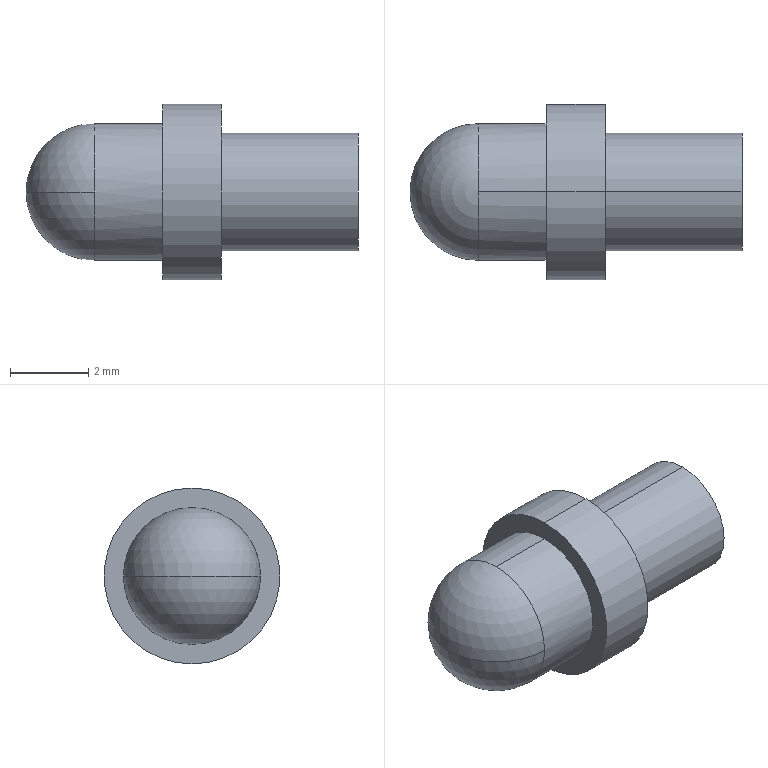Part | STEP file | RSR-PB107_grease_nipple_joint(2)^SRS15MUU-220LM-G10_Buffer motion shaft | 1 solid | 11 faces | box 8.5 x 4.5 x 4.5 mm | volume 76.658 mm3 | cylinder 6 | plane 3 | sphere 2 | commonest cylinder face diameters 3 x2 3.5 x2 4.5 x2
STEP:
#1=CARTESIAN_POINT('',(0.,0.,0.));
#2=DIRECTION('',(0.,0.,1.));
#3=DIRECTION('',(1.,0.,0.));
#4=AXIS2_PLACEMENT_3D('',#1,#2,#3);
#5=CARTESIAN_POINT('',(-5.,0.,0.));
#6=VERTEX_POINT('',#5);
#7=CARTESIAN_POINT('',(-3.25,1.75,0.));
#8=VERTEX_POINT('',#7);
#9=CARTESIAN_POINT('',(-3.25,0.,0.));
#10=DIRECTION('',(0.,0.,-1.));
#11=DIRECTION('',(-1.,0.,0.));
#12=AXIS2_PLACEMENT_3D('',#9,#10,#11);
#13=CIRCLE('',#12,1.75);
#14=CARTESIAN_POINT('',(-3.25,0.,0.));
#15=DIRECTION('',(0.,0.,1.));
#16=DIRECTION('',(0.,1.,0.));
#17=AXIS2_PLACEMENT_3D('',#14,#15,#16);
#18=SPHERICAL_SURFACE('',#17,1.75);
#19=CARTESIAN_POINT('',(1.571,0.));
#20=DIRECTION('',(-1.,0.));
#21=VECTOR('',#20,1.);
#22=LINE('',#19,#21);
#23=(GEOMETRIC_REPRESENTATION_CONTEXT(2)PARAMETRIC_REPRESENTATION_CONTEXT()REPRESENTATION_CONTEXT('',''));
#24=DEFINITIONAL_REPRESENTATION('',(#22),#23);
#25=PCURVE('',#18,#24);
#26=CARTESIAN_POINT('',(-3.25,0.,0.));
#27=DIRECTION('',(0.,0.,1.));
#28=DIRECTION('',(0.,1.,0.));
#29=AXIS2_PLACEMENT_3D('',#26,#27,#28);
#30=SPHERICAL_SURFACE('',#29,1.75);
#31=CARTESIAN_POINT('',(1.571,0.));
#32=DIRECTION('',(-1.,0.));
#33=VECTOR('',#32,1.);
#34=LINE('',#31,#33);
#35=(GEOMETRIC_REPRESENTATION_CONTEXT(2)PARAMETRIC_REPRESENTATION_CONTEXT()REPRESENTATION_CONTEXT('',''));
#36=DEFINITIONAL_REPRESENTATION('',(#34),#35);
#37=PCURVE('',#30,#36);
#38=SURFACE_CURVE('',#13,(#25,#37),.PCURVE_S1.);
#39=EDGE_CURVE('',#6,#8,#38,.T.);
#40=ORIENTED_EDGE('',*,*,#39,.F.);
#41=CARTESIAN_POINT('',(-3.25,-1.75,0.));
#42=VERTEX_POINT('',#41);
#43=CARTESIAN_POINT('',(-3.25,0.,0.));
#44=DIRECTION('',(0.,0.,1.));
#45=DIRECTION('',(0.,-1.,0.));
#46=AXIS2_PLACEMENT_3D('',#43,#44,#45);
#47=CIRCLE('',#46,1.75);
#48=CARTESIAN_POINT('',(-3.142,0.));
#49=DIRECTION('',(1.,0.));
#50=VECTOR('',#49,1.);
#51=LINE('',#48,#50);
#52=(GEOMETRIC_REPRESENTATION_CONTEXT(2)PARAMETRIC_REPRESENTATION_CONTEXT()REPRESENTATION_CONTEXT('',''));
#53=DEFINITIONAL_REPRESENTATION('',(#51),#52);
#54=PCURVE('',#18,#53);
#55=CARTESIAN_POINT('',(-3.142,0.));
#56=DIRECTION('',(1.,0.));
#57=VECTOR('',#56,1.);
#58=LINE('',#55,#57);
#59=(GEOMETRIC_REPRESENTATION_CONTEXT(2)PARAMETRIC_REPRESENTATION_CONTEXT()REPRESENTATION_CONTEXT('',''));
#60=DEFINITIONAL_REPRESENTATION('',(#58),#59);
#61=PCURVE('',#30,#60);
#62=SURFACE_CURVE('',#47,(#54,#61),.PCURVE_S1.);
#63=EDGE_CURVE('',#6,#42,#62,.T.);
#64=ORIENTED_EDGE('',*,*,#63,.T.);
#65=CARTESIAN_POINT('',(-3.25,0.,1.75));
#66=VERTEX_POINT('',#65);
#67=CARTESIAN_POINT('',(-3.25,0.,0.));
#68=DIRECTION('',(1.,0.,0.));
#69=DIRECTION('',(0.,0.,-1.));
#70=AXIS2_PLACEMENT_3D('',#67,#68,#69);
#71=CIRCLE('',#70,1.75);
#72=CARTESIAN_POINT('',(3.142,1.571));
#73=CARTESIAN_POINT('',(3.142,1.547));
#74=CARTESIAN_POINT('',(3.142,1.499));
#75=CARTESIAN_POINT('',(3.142,1.428));
#76=CARTESIAN_POINT('',(3.142,1.357));
#77=CARTESIAN_POINT('',(3.142,1.285));
#78=CARTESIAN_POINT('',(3.142,1.214));
#79=CARTESIAN_POINT('',(3.142,1.142));
#80=CARTESIAN_POINT('',(3.142,1.071));
#81=CARTESIAN_POINT('',(3.142,0.9996));
#82=CARTESIAN_POINT('',(3.142,0.9282));
#83=CARTESIAN_POINT('',(3.142,0.8568));
#84=CARTESIAN_POINT('',(3.142,0.7854));
#85=CARTESIAN_POINT('',(3.142,0.714));
#86=CARTESIAN_POINT('',(3.142,0.6426));
#87=CARTESIAN_POINT('',(3.142,0.5712));
#88=CARTESIAN_POINT('',(3.142,0.4998));
#89=CARTESIAN_POINT('',(3.142,0.4284));
#90=CARTESIAN_POINT('',(3.142,0.357));
#91=CARTESIAN_POINT('',(3.142,0.2856));
#92=CARTESIAN_POINT('',(3.142,0.2142));
#93=CARTESIAN_POINT('',(3.142,0.1428));
#94=CARTESIAN_POINT('',(3.142,0.0714));
#95=CARTESIAN_POINT('',(3.142,0.0238));
#96=CARTESIAN_POINT('',(3.142,0.));
#97=B_SPLINE_CURVE_WITH_KNOTS('',3,(#72,#73,#74,#75,#76,#77,#78,#79,#80,#81,#82,#83,#84,#85,#86,#87,#88,#89,#90,#91,#92,#93,#94,#95,#96),.UNSPECIFIED.,.F.,.F.,(4,1,1,1,1,1,1,1,1,1,1,1,1,1,1,1,1,1,1,1,1,1,4),(3.142,3.213,3.284,3.356,3.427,3.499,3.57,3.641,3.713,3.784,3.856,3.927,3.998,4.07,4.141,4.213,4.284,4.355,4.427,4.498,4.57,4.641,4.712),.QUASI_UNIFORM_KNOTS.);
#98=(GEOMETRIC_REPRESENTATION_CONTEXT(2)PARAMETRIC_REPRESENTATION_CONTEXT()REPRESENTATION_CONTEXT('',''));
#99=DEFINITIONAL_REPRESENTATION('',(#97),#98);
#100=PCURVE('',#18,#99);
#101=CARTESIAN_POINT('',(3.5,0.,0.));
#102=DIRECTION('',(1.,0.,0.));
#103=DIRECTION('',(0.,0.,-1.));
#104=AXIS2_PLACEMENT_3D('',#101,#102,#103);
#105=CYLINDRICAL_SURFACE('',#104,1.75);
#106=CARTESIAN_POINT('',(0.,-6.75));
#107=DIRECTION('',(1.,0.));
#108=VECTOR('',#107,1.);
#109=LINE('',#106,#108);
#110=(GEOMETRIC_REPRESENTATION_CONTEXT(2)PARAMETRIC_REPRESENTATION_CONTEXT()REPRESENTATION_CONTEXT('',''));
#111=DEFINITIONAL_REPRESENTATION('',(#109),#110);
#112=PCURVE('',#105,#111);
#113=SURFACE_CURVE('',#71,(#100,#112),.PCURVE_S1.);
#114=EDGE_CURVE('',#66,#42,#113,.T.);
#115=ORIENTED_EDGE('',*,*,#114,.F.);
#116=CARTESIAN_POINT('',(-3.25,0.,0.));
#117=DIRECTION('',(1.,0.,0.));
#118=DIRECTION('',(0.,0.,-1.));
#119=AXIS2_PLACEMENT_3D('',#116,#117,#118);
#120=CIRCLE('',#119,1.75);
#121=CARTESIAN_POINT('',(0.,-1.571));
#122=DIRECTION('',(0.,1.));
#123=VECTOR('',#122,1.);
#124=LINE('',#121,#123);
#125=(GEOMETRIC_REPRESENTATION_CONTEXT(2)PARAMETRIC_REPRESENTATION_CONTEXT()REPRESENTATION_CONTEXT('',''));
#126=DEFINITIONAL_REPRESENTATION('',(#124),#125);
#127=PCURVE('',#18,#126);
#128=CARTESIAN_POINT('',(3.5,0.,0.));
#129=DIRECTION('',(1.,0.,0.));
#130=DIRECTION('',(0.,0.,-1.));
#131=AXIS2_PLACEMENT_3D('',#128,#129,#130);
#132=CYLINDRICAL_SURFACE('',#131,1.75);
#133=CARTESIAN_POINT('',(0.,-6.75));
#134=DIRECTION('',(1.,0.));
#135=VECTOR('',#134,1.);
#136=LINE('',#133,#135);
#137=(GEOMETRIC_REPRESENTATION_CONTEXT(2)PARAMETRIC_REPRESENTATION_CONTEXT()REPRESENTATION_CONTEXT('',''));
#138=DEFINITIONAL_REPRESENTATION('',(#136),#137);
#139=PCURVE('',#132,#138);
#140=SURFACE_CURVE('',#120,(#127,#139),.PCURVE_S1.);
#141=EDGE_CURVE('',#8,#66,#140,.T.);
#142=ORIENTED_EDGE('',*,*,#141,.F.);
#143=EDGE_LOOP('',(#40,#64,#115,#142));
#144=FACE_BOUND('',#143,.T.);
#145=ADVANCED_FACE('',(#144),#18,.T.);
#146=CARTESIAN_POINT('',(-3.25,0.,-1.75));
#147=VERTEX_POINT('',#146);
#148=CARTESIAN_POINT('',(-3.25,0.,0.));
#149=DIRECTION('',(1.,0.,0.));
#150=DIRECTION('',(0.,0.,-1.));
#151=AXIS2_PLACEMENT_3D('',#148,#149,#150);
#152=CIRCLE('',#151,1.75);
#153=CARTESIAN_POINT('',(0.,-6.75));
#154=DIRECTION('',(1.,0.));
#155=VECTOR('',#154,1.);
#156=LINE('',#153,#155);
#157=(GEOMETRIC_REPRESENTATION_CONTEXT(2)PARAMETRIC_REPRESENTATION_CONTEXT()REPRESENTATION_CONTEXT('',''));
#158=DEFINITIONAL_REPRESENTATION('',(#156),#157);
#159=PCURVE('',#132,#158);
#160=CARTESIAN_POINT('',(0.,-1.571));
#161=DIRECTION('',(0.,1.));
#162=VECTOR('',#161,1.);
#163=LINE('',#160,#162);
#164=(GEOMETRIC_REPRESENTATION_CONTEXT(2)PARAMETRIC_REPRESENTATION_CONTEXT()REPRESENTATION_CONTEXT('',''));
#165=DEFINITIONAL_REPRESENTATION('',(#163),#164);
#166=PCURVE('',#30,#165);
#167=SURFACE_CURVE('',#152,(#159,#166),.PCURVE_S1.);
#168=EDGE_CURVE('',#147,#8,#167,.T.);
#169=ORIENTED_EDGE('',*,*,#168,.T.);
#170=ORIENTED_EDGE('',*,*,#141,.T.);
#171=CARTESIAN_POINT('',(-1.5,0.,1.75));
#172=VERTEX_POINT('',#171);
#173=CARTESIAN_POINT('',(3.5,0.,1.75));
#174=DIRECTION('',(1.,0.,0.));
#175=VECTOR('',#174,1.);
#176=LINE('',#173,#175);
#177=CARTESIAN_POINT('',(3.142,0.));
#178=DIRECTION('',(0.,1.));
#179=VECTOR('',#178,1.);
#180=LINE('',#177,#179);
#181=(GEOMETRIC_REPRESENTATION_CONTEXT(2)PARAMETRIC_REPRESENTATION_CONTEXT()REPRESENTATION_CONTEXT('',''));
#182=DEFINITIONAL_REPRESENTATION('',(#180),#181);
#183=PCURVE('',#132,#182);
#184=CARTESIAN_POINT('',(3.142,0.));
#185=DIRECTION('',(0.,1.));
#186=VECTOR('',#185,1.);
#187=LINE('',#184,#186);
#188=(GEOMETRIC_REPRESENTATION_CONTEXT(2)PARAMETRIC_REPRESENTATION_CONTEXT()REPRESENTATION_CONTEXT('',''));
#189=DEFINITIONAL_REPRESENTATION('',(#187),#188);
#190=PCURVE('',#105,#189);
#191=SURFACE_CURVE('',#176,(#183,#190),.PCURVE_S1.);
#192=EDGE_CURVE('',#66,#172,#191,.T.);
#193=ORIENTED_EDGE('',*,*,#192,.T.);
#194=CARTESIAN_POINT('',(-1.5,0.,-1.75));
#195=VERTEX_POINT('',#194);
#196=CARTESIAN_POINT('',(-1.5,0.,0.));
#197=DIRECTION('',(1.,0.,0.));
#198=DIRECTION('',(0.,0.,-1.));
#199=AXIS2_PLACEMENT_3D('',#196,#197,#198);
#200=CIRCLE('',#199,1.75);
#201=CARTESIAN_POINT('',(0.,-5.));
#202=DIRECTION('',(1.,0.));
#203=VECTOR('',#202,1.);
#204=LINE('',#201,#203);
#205=(GEOMETRIC_REPRESENTATION_CONTEXT(2)PARAMETRIC_REPRESENTATION_CONTEXT()REPRESENTATION_CONTEXT('',''));
#206=DEFINITIONAL_REPRESENTATION('',(#204),#205);
#207=PCURVE('',#132,#206);
#208=CARTESIAN_POINT('',(-1.5,1.75,0.));
#209=DIRECTION('',(1.,0.,0.));
#210=DIRECTION('',(0.,1.,0.));
#211=AXIS2_PLACEMENT_3D('',#208,#209,#210);
#212=PLANE('',#211);
#213=CARTESIAN_POINT('',(-1.75,0.));
#214=DIRECTION('',(0.,-1.));
#215=AXIS2_PLACEMENT_2D('',#213,#214);
#216=CIRCLE('',#215,1.75);
#217=(GEOMETRIC_REPRESENTATION_CONTEXT(2)PARAMETRIC_REPRESENTATION_CONTEXT()REPRESENTATION_CONTEXT('',''));
#218=DEFINITIONAL_REPRESENTATION('',(#216),#217);
#219=PCURVE('',#212,#218);
#220=SURFACE_CURVE('',#200,(#207,#219),.PCURVE_S1.);
#221=EDGE_CURVE('',#195,#172,#220,.T.);
#222=ORIENTED_EDGE('',*,*,#221,.F.);
#223=CARTESIAN_POINT('',(3.5,0.,-1.75));
#224=DIRECTION('',(1.,0.,0.));
#225=VECTOR('',#224,1.);
#226=LINE('',#223,#225);
#227=CARTESIAN_POINT('',(0.,0.));
#228=DIRECTION('',(0.,1.));
#229=VECTOR('',#228,1.);
#230=LINE('',#227,#229);
#231=(GEOMETRIC_REPRESENTATION_CONTEXT(2)PARAMETRIC_REPRESENTATION_CONTEXT()REPRESENTATION_CONTEXT('',''));
#232=DEFINITIONAL_REPRESENTATION('',(#230),#231);
#233=PCURVE('',#132,#232);
#234=CARTESIAN_POINT('',(6.283,0.));
#235=DIRECTION('',(0.,1.));
#236=VECTOR('',#235,1.);
#237=LINE('',#234,#236);
#238=(GEOMETRIC_REPRESENTATION_CONTEXT(2)PARAMETRIC_REPRESENTATION_CONTEXT()REPRESENTATION_CONTEXT('',''));
#239=DEFINITIONAL_REPRESENTATION('',(#237),#238);
#240=PCURVE('',#105,#239);
#241=SURFACE_CURVE('',#226,(#233,#240),.PCURVE_S1.);
#242=EDGE_CURVE('',#147,#195,#241,.T.);
#243=ORIENTED_EDGE('',*,*,#242,.F.);
#244=EDGE_LOOP('',(#169,#170,#193,#222,#243));
#245=FACE_BOUND('',#244,.T.);
#246=ADVANCED_FACE('',(#245),#132,.T.);
#247=CARTESIAN_POINT('',(-1.5,0.,-2.25));
#248=VERTEX_POINT('',#247);
#249=CARTESIAN_POINT('',(-1.5,0.,2.25));
#250=VERTEX_POINT('',#249);
#251=CARTESIAN_POINT('',(-1.5,0.,0.));
#252=DIRECTION('',(1.,0.,0.));
#253=DIRECTION('',(0.,0.,-1.));
#254=AXIS2_PLACEMENT_3D('',#251,#252,#253);
#255=CIRCLE('',#254,2.25);
#256=CARTESIAN_POINT('',(3.5,0.,0.));
#257=DIRECTION('',(1.,0.,0.));
#258=DIRECTION('',(0.,0.,-1.));
#259=AXIS2_PLACEMENT_3D('',#256,#257,#258);
#260=CYLINDRICAL_SURFACE('',#259,2.25);
#261=CARTESIAN_POINT('',(0.,-5.));
#262=DIRECTION('',(1.,0.));
#263=VECTOR('',#262,1.);
#264=LINE('',#261,#263);
#265=(GEOMETRIC_REPRESENTATION_CONTEXT(2)PARAMETRIC_REPRESENTATION_CONTEXT()REPRESENTATION_CONTEXT('',''));
#266=DEFINITIONAL_REPRESENTATION('',(#264),#265);
#267=PCURVE('',#260,#266);
#268=CARTESIAN_POINT('',(-1.75,0.));
#269=DIRECTION('',(0.,-1.));
#270=AXIS2_PLACEMENT_2D('',#268,#269);
#271=CIRCLE('',#270,2.25);
#272=(GEOMETRIC_REPRESENTATION_CONTEXT(2)PARAMETRIC_REPRESENTATION_CONTEXT()REPRESENTATION_CONTEXT('',''));
#273=DEFINITIONAL_REPRESENTATION('',(#271),#272);
#274=PCURVE('',#212,#273);
#275=SURFACE_CURVE('',#255,(#267,#274),.PCURVE_S1.);
#276=EDGE_CURVE('',#248,#250,#275,.T.);
#277=ORIENTED_EDGE('',*,*,#276,.T.);
#278=CARTESIAN_POINT('',(0.,0.,2.25));
#279=VERTEX_POINT('',#278);
#280=CARTESIAN_POINT('',(3.5,0.,2.25));
#281=DIRECTION('',(1.,0.,0.));
#282=VECTOR('',#281,1.);
#283=LINE('',#280,#282);
#284=CARTESIAN_POINT('',(3.142,0.));
#285=DIRECTION('',(0.,1.));
#286=VECTOR('',#285,1.);
#287=LINE('',#284,#286);
#288=(GEOMETRIC_REPRESENTATION_CONTEXT(2)PARAMETRIC_REPRESENTATION_CONTEXT()REPRESENTATION_CONTEXT('',''));
#289=DEFINITIONAL_REPRESENTATION('',(#287),#288);
#290=PCURVE('',#260,#289);
#291=CARTESIAN_POINT('',(3.5,0.,0.));
#292=DIRECTION('',(1.,0.,0.));
#293=DIRECTION('',(0.,0.,-1.));
#294=AXIS2_PLACEMENT_3D('',#291,#292,#293);
#295=CYLINDRICAL_SURFACE('',#294,2.25);
#296=CARTESIAN_POINT('',(3.142,0.));
#297=DIRECTION('',(0.,1.));
#298=VECTOR('',#297,1.);
#299=LINE('',#296,#298);
#300=(GEOMETRIC_REPRESENTATION_CONTEXT(2)PARAMETRIC_REPRESENTATION_CONTEXT()REPRESENTATION_CONTEXT('',''));
#301=DEFINITIONAL_REPRESENTATION('',(#299),#300);
#302=PCURVE('',#295,#301);
#303=SURFACE_CURVE('',#283,(#290,#302),.PCURVE_S1.);
#304=EDGE_CURVE('',#250,#279,#303,.T.);
#305=ORIENTED_EDGE('',*,*,#304,.T.);
#306=CARTESIAN_POINT('',(0.,0.,-2.25));
#307=VERTEX_POINT('',#306);
#308=CARTESIAN_POINT('',(0.,0.,0.));
#309=DIRECTION('',(1.,0.,0.));
#310=DIRECTION('',(0.,0.,-1.));
#311=AXIS2_PLACEMENT_3D('',#308,#309,#310);
#312=CIRCLE('',#311,2.25);
#313=CARTESIAN_POINT('',(0.,-3.5));
#314=DIRECTION('',(1.,0.));
#315=VECTOR('',#314,1.);
#316=LINE('',#313,#315);
#317=(GEOMETRIC_REPRESENTATION_CONTEXT(2)PARAMETRIC_REPRESENTATION_CONTEXT()REPRESENTATION_CONTEXT('',''));
#318=DEFINITIONAL_REPRESENTATION('',(#316),#317);
#319=PCURVE('',#260,#318);
#320=CARTESIAN_POINT('',(0.,2.25,0.));
#321=DIRECTION('',(-1.,0.,0.));
#322=DIRECTION('',(0.,0.,1.));
#323=AXIS2_PLACEMENT_3D('',#320,#321,#322);
#324=PLANE('',#323);
#325=CARTESIAN_POINT('',(-2.25,-2.25));
#326=CARTESIAN_POINT('',(-2.25,1.647));
#327=CARTESIAN_POINT('',(1.125,-0.3014));
#328=CARTESIAN_POINT('',(4.5,-2.25));
#329=CARTESIAN_POINT('',(1.125,-4.199));
#330=CARTESIAN_POINT('',(-2.25,-6.147));
#331=CARTESIAN_POINT('',(-2.25,-2.25));
#332=(BOUNDED_CURVE()B_SPLINE_CURVE(2,(#325,#326,#327,#328,#329,#330,#331),.UNSPECIFIED.,.T.,.F.)B_SPLINE_CURVE_WITH_KNOTS((1,2,2,2,2,1),(-2.094,0.,2.094,4.189,6.283,8.378),.UNSPECIFIED.)CURVE()GEOMETRIC_REPRESENTATION_ITEM()RATIONAL_B_SPLINE_CURVE((1.,0.5,1.,0.5,1.,0.5,1.))REPRESENTATION_ITEM(''));
#333=(GEOMETRIC_REPRESENTATION_CONTEXT(2)PARAMETRIC_REPRESENTATION_CONTEXT()REPRESENTATION_CONTEXT('',''));
#334=DEFINITIONAL_REPRESENTATION('',(#332),#333);
#335=PCURVE('',#324,#334);
#336=SURFACE_CURVE('',#312,(#319,#335),.PCURVE_S1.);
#337=EDGE_CURVE('',#307,#279,#336,.T.);
#338=ORIENTED_EDGE('',*,*,#337,.F.);
#339=CARTESIAN_POINT('',(3.5,0.,-2.25));
#340=DIRECTION('',(1.,0.,0.));
#341=VECTOR('',#340,1.);
#342=LINE('',#339,#341);
#343=CARTESIAN_POINT('',(0.,0.));
#344=DIRECTION('',(0.,1.));
#345=VECTOR('',#344,1.);
#346=LINE('',#343,#345);
#347=(GEOMETRIC_REPRESENTATION_CONTEXT(2)PARAMETRIC_REPRESENTATION_CONTEXT()REPRESENTATION_CONTEXT('',''));
#348=DEFINITIONAL_REPRESENTATION('',(#346),#347);
#349=PCURVE('',#260,#348);
#350=CARTESIAN_POINT('',(6.283,0.));
#351=DIRECTION('',(0.,1.));
#352=VECTOR('',#351,1.);
#353=LINE('',#350,#352);
#354=(GEOMETRIC_REPRESENTATION_CONTEXT(2)PARAMETRIC_REPRESENTATION_CONTEXT()REPRESENTATION_CONTEXT('',''));
#355=DEFINITIONAL_REPRESENTATION('',(#353),#354);
#356=PCURVE('',#295,#355);
#357=SURFACE_CURVE('',#342,(#349,#356),.PCURVE_S1.);
#358=EDGE_CURVE('',#248,#307,#357,.T.);
#359=ORIENTED_EDGE('',*,*,#358,.F.);
#360=EDGE_LOOP('',(#277,#305,#338,#359));
#361=FACE_BOUND('',#360,.T.);
#362=ADVANCED_FACE('',(#361),#260,.T.);
#363=CARTESIAN_POINT('',(0.,0.,-1.5));
#364=VERTEX_POINT('',#363);
#365=CARTESIAN_POINT('',(0.,0.,1.5));
#366=VERTEX_POINT('',#365);
#367=CARTESIAN_POINT('',(0.,0.,0.));
#368=DIRECTION('',(1.,0.,0.));
#369=DIRECTION('',(0.,0.,-1.));
#370=AXIS2_PLACEMENT_3D('',#367,#368,#369);
#371=CIRCLE('',#370,1.5);
#372=CARTESIAN_POINT('',(3.5,0.,0.));
#373=DIRECTION('',(1.,0.,0.));
#374=DIRECTION('',(0.,0.,-1.));
#375=AXIS2_PLACEMENT_3D('',#372,#373,#374);
#376=CYLINDRICAL_SURFACE('',#375,1.5);
#377=CARTESIAN_POINT('',(0.,-3.5));
#378=DIRECTION('',(1.,0.));
#379=VECTOR('',#378,1.);
#380=LINE('',#377,#379);
#381=(GEOMETRIC_REPRESENTATION_CONTEXT(2)PARAMETRIC_REPRESENTATION_CONTEXT()REPRESENTATION_CONTEXT('',''));
#382=DEFINITIONAL_REPRESENTATION('',(#380),#381);
#383=PCURVE('',#376,#382);
#384=CARTESIAN_POINT('',(-1.5,-2.25));
#385=CARTESIAN_POINT('',(-1.5,0.3481));
#386=CARTESIAN_POINT('',(0.75,-0.951));
#387=CARTESIAN_POINT('',(3.,-2.25));
#388=CARTESIAN_POINT('',(0.75,-3.549));
#389=CARTESIAN_POINT('',(-1.5,-4.848));
#390=CARTESIAN_POINT('',(-1.5,-2.25));
#391=(BOUNDED_CURVE()B_SPLINE_CURVE(2,(#384,#385,#386,#387,#388,#389,#390),.UNSPECIFIED.,.T.,.F.)B_SPLINE_CURVE_WITH_KNOTS((1,2,2,2,2,1),(-2.094,0.,2.094,4.189,6.283,8.378),.UNSPECIFIED.)CURVE()GEOMETRIC_REPRESENTATION_ITEM()RATIONAL_B_SPLINE_CURVE((1.,0.5,1.,0.5,1.,0.5,1.))REPRESENTATION_ITEM(''));
#392=(GEOMETRIC_REPRESENTATION_CONTEXT(2)PARAMETRIC_REPRESENTATION_CONTEXT()REPRESENTATION_CONTEXT('',''));
#393=DEFINITIONAL_REPRESENTATION('',(#391),#392);
#394=PCURVE('',#324,#393);
#395=SURFACE_CURVE('',#371,(#383,#394),.PCURVE_S1.);
#396=EDGE_CURVE('',#364,#366,#395,.T.);
#397=ORIENTED_EDGE('',*,*,#396,.T.);
#398=CARTESIAN_POINT('',(3.5,0.,1.5));
#399=VERTEX_POINT('',#398);
#400=CARTESIAN_POINT('',(3.5,0.,1.5));
#401=DIRECTION('',(1.,0.,0.));
#402=VECTOR('',#401,1.);
#403=LINE('',#400,#402);
#404=CARTESIAN_POINT('',(3.142,0.));
#405=DIRECTION('',(0.,1.));
#406=VECTOR('',#405,1.);
#407=LINE('',#404,#406);
#408=(GEOMETRIC_REPRESENTATION_CONTEXT(2)PARAMETRIC_REPRESENTATION_CONTEXT()REPRESENTATION_CONTEXT('',''));
#409=DEFINITIONAL_REPRESENTATION('',(#407),#408);
#410=PCURVE('',#376,#409);
#411=CARTESIAN_POINT('',(3.5,0.,0.));
#412=DIRECTION('',(1.,0.,0.));
#413=DIRECTION('',(0.,0.,-1.));
#414=AXIS2_PLACEMENT_3D('',#411,#412,#413);
#415=CYLINDRICAL_SURFACE('',#414,1.5);
#416=CARTESIAN_POINT('',(3.142,0.));
#417=DIRECTION('',(0.,1.));
#418=VECTOR('',#417,1.);
#419=LINE('',#416,#418);
#420=(GEOMETRIC_REPRESENTATION_CONTEXT(2)PARAMETRIC_REPRESENTATION_CONTEXT()REPRESENTATION_CONTEXT('',''));
#421=DEFINITIONAL_REPRESENTATION('',(#419),#420);
#422=PCURVE('',#415,#421);
#423=SURFACE_CURVE('',#403,(#410,#422),.PCURVE_S1.);
#424=EDGE_CURVE('',#366,#399,#423,.T.);
#425=ORIENTED_EDGE('',*,*,#424,.T.);
#426=CARTESIAN_POINT('',(3.5,0.,-1.5));
#427=VERTEX_POINT('',#426);
#428=CARTESIAN_POINT('',(3.5,0.,0.));
#429=DIRECTION('',(1.,0.,0.));
#430=DIRECTION('',(0.,0.,-1.));
#431=AXIS2_PLACEMENT_3D('',#428,#429,#430);
#432=CIRCLE('',#431,1.5);
#433=CARTESIAN_POINT('',(0.,0.));
#434=DIRECTION('',(1.,0.));
#435=VECTOR('',#434,1.);
#436=LINE('',#433,#435);
#437=(GEOMETRIC_REPRESENTATION_CONTEXT(2)PARAMETRIC_REPRESENTATION_CONTEXT()REPRESENTATION_CONTEXT('',''));
#438=DEFINITIONAL_REPRESENTATION('',(#436),#437);
#439=PCURVE('',#376,#438);
#440=CARTESIAN_POINT('',(3.5,1.5,0.));
#441=DIRECTION('',(-1.,0.,0.));
#442=DIRECTION('',(0.,0.,1.));
#443=AXIS2_PLACEMENT_3D('',#440,#441,#442);
#444=PLANE('',#443);
#445=CARTESIAN_POINT('',(-1.5,-1.5));
#446=CARTESIAN_POINT('',(-1.5,1.098));
#447=CARTESIAN_POINT('',(0.75,-0.201));
#448=CARTESIAN_POINT('',(3.,-1.5));
#449=CARTESIAN_POINT('',(0.75,-2.799));
#450=CARTESIAN_POINT('',(-1.5,-4.098));
#451=CARTESIAN_POINT('',(-1.5,-1.5));
#452=(BOUNDED_CURVE()B_SPLINE_CURVE(2,(#445,#446,#447,#448,#449,#450,#451),.UNSPECIFIED.,.T.,.F.)B_SPLINE_CURVE_WITH_KNOTS((1,2,2,2,2,1),(-2.094,0.,2.094,4.189,6.283,8.378),.UNSPECIFIED.)CURVE()GEOMETRIC_REPRESENTATION_ITEM()RATIONAL_B_SPLINE_CURVE((1.,0.5,1.,0.5,1.,0.5,1.))REPRESENTATION_ITEM(''));
#453=(GEOMETRIC_REPRESENTATION_CONTEXT(2)PARAMETRIC_REPRESENTATION_CONTEXT()REPRESENTATION_CONTEXT('',''));
#454=DEFINITIONAL_REPRESENTATION('',(#452),#453);
#455=PCURVE('',#444,#454);
#456=SURFACE_CURVE('',#432,(#439,#455),.PCURVE_S1.);
#457=EDGE_CURVE('',#427,#399,#456,.T.);
#458=ORIENTED_EDGE('',*,*,#457,.F.);
#459=CARTESIAN_POINT('',(3.5,0.,-1.5));
#460=DIRECTION('',(1.,0.,0.));
#461=VECTOR('',#460,1.);
#462=LINE('',#459,#461);
#463=CARTESIAN_POINT('',(0.,0.));
#464=DIRECTION('',(0.,1.));
#465=VECTOR('',#464,1.);
#466=LINE('',#463,#465);
#467=(GEOMETRIC_REPRESENTATION_CONTEXT(2)PARAMETRIC_REPRESENTATION_CONTEXT()REPRESENTATION_CONTEXT('',''));
#468=DEFINITIONAL_REPRESENTATION('',(#466),#467);
#469=PCURVE('',#376,#468);
#470=CARTESIAN_POINT('',(6.283,0.));
#471=DIRECTION('',(0.,1.));
#472=VECTOR('',#471,1.);
#473=LINE('',#470,#472);
#474=(GEOMETRIC_REPRESENTATION_CONTEXT(2)PARAMETRIC_REPRESENTATION_CONTEXT()REPRESENTATION_CONTEXT('',''));
#475=DEFINITIONAL_REPRESENTATION('',(#473),#474);
#476=PCURVE('',#415,#475);
#477=SURFACE_CURVE('',#462,(#469,#476),.PCURVE_S1.);
#478=EDGE_CURVE('',#364,#427,#477,.T.);
#479=ORIENTED_EDGE('',*,*,#478,.F.);
#480=EDGE_LOOP('',(#397,#425,#458,#479));
#481=FACE_BOUND('',#480,.T.);
#482=ADVANCED_FACE('',(#481),#376,.T.);
#483=ORIENTED_EDGE('',*,*,#457,.T.);
#484=CARTESIAN_POINT('',(3.5,0.,0.));
#485=DIRECTION('',(1.,0.,0.));
#486=DIRECTION('',(0.,0.,-1.));
#487=AXIS2_PLACEMENT_3D('',#484,#485,#486);
#488=CIRCLE('',#487,1.5);
#489=CARTESIAN_POINT('',(-1.5,-1.5));
#490=CARTESIAN_POINT('',(-1.5,1.098));
#491=CARTESIAN_POINT('',(0.75,-0.201));
#492=CARTESIAN_POINT('',(3.,-1.5));
#493=CARTESIAN_POINT('',(0.75,-2.799));
#494=CARTESIAN_POINT('',(-1.5,-4.098));
#495=CARTESIAN_POINT('',(-1.5,-1.5));
#496=(BOUNDED_CURVE()B_SPLINE_CURVE(2,(#489,#490,#491,#492,#493,#494,#495),.UNSPECIFIED.,.T.,.F.)B_SPLINE_CURVE_WITH_KNOTS((1,2,2,2,2,1),(-2.094,0.,2.094,4.189,6.283,8.378),.UNSPECIFIED.)CURVE()GEOMETRIC_REPRESENTATION_ITEM()RATIONAL_B_SPLINE_CURVE((1.,0.5,1.,0.5,1.,0.5,1.))REPRESENTATION_ITEM(''));
#497=(GEOMETRIC_REPRESENTATION_CONTEXT(2)PARAMETRIC_REPRESENTATION_CONTEXT()REPRESENTATION_CONTEXT('',''));
#498=DEFINITIONAL_REPRESENTATION('',(#496),#497);
#499=PCURVE('',#444,#498);
#500=CARTESIAN_POINT('',(0.,0.));
#501=DIRECTION('',(1.,0.));
#502=VECTOR('',#501,1.);
#503=LINE('',#500,#502);
#504=(GEOMETRIC_REPRESENTATION_CONTEXT(2)PARAMETRIC_REPRESENTATION_CONTEXT()REPRESENTATION_CONTEXT('',''));
#505=DEFINITIONAL_REPRESENTATION('',(#503),#504);
#506=PCURVE('',#415,#505);
#507=SURFACE_CURVE('',#488,(#499,#506),.PCURVE_S1.);
#508=EDGE_CURVE('',#399,#427,#507,.T.);
#509=ORIENTED_EDGE('',*,*,#508,.T.);
#510=EDGE_LOOP('',(#483,#509));
#511=FACE_BOUND('',#510,.T.);
#512=ADVANCED_FACE('',(#511),#444,.F.);
#513=ORIENTED_EDGE('',*,*,#424,.F.);
#514=CARTESIAN_POINT('',(0.,0.,0.));
#515=DIRECTION('',(1.,0.,0.));
#516=DIRECTION('',(0.,0.,-1.));
#517=AXIS2_PLACEMENT_3D('',#514,#515,#516);
#518=CIRCLE('',#517,1.5);
#519=CARTESIAN_POINT('',(0.,-3.5));
#520=DIRECTION('',(1.,0.));
#521=VECTOR('',#520,1.);
#522=LINE('',#519,#521);
#523=(GEOMETRIC_REPRESENTATION_CONTEXT(2)PARAMETRIC_REPRESENTATION_CONTEXT()REPRESENTATION_CONTEXT('',''));
#524=DEFINITIONAL_REPRESENTATION('',(#522),#523);
#525=PCURVE('',#415,#524);
#526=CARTESIAN_POINT('',(-1.5,-2.25));
#527=CARTESIAN_POINT('',(-1.5,0.3481));
#528=CARTESIAN_POINT('',(0.75,-0.951));
#529=CARTESIAN_POINT('',(3.,-2.25));
#530=CARTESIAN_POINT('',(0.75,-3.549));
#531=CARTESIAN_POINT('',(-1.5,-4.848));
#532=CARTESIAN_POINT('',(-1.5,-2.25));
#533=(BOUNDED_CURVE()B_SPLINE_CURVE(2,(#526,#527,#528,#529,#530,#531,#532),.UNSPECIFIED.,.T.,.F.)B_SPLINE_CURVE_WITH_KNOTS((1,2,2,2,2,1),(-2.094,0.,2.094,4.189,6.283,8.378),.UNSPECIFIED.)CURVE()GEOMETRIC_REPRESENTATION_ITEM()RATIONAL_B_SPLINE_CURVE((1.,0.5,1.,0.5,1.,0.5,1.))REPRESENTATION_ITEM(''));
#534=(GEOMETRIC_REPRESENTATION_CONTEXT(2)PARAMETRIC_REPRESENTATION_CONTEXT()REPRESENTATION_CONTEXT('',''));
#535=DEFINITIONAL_REPRESENTATION('',(#533),#534);
#536=PCURVE('',#324,#535);
#537=SURFACE_CURVE('',#518,(#525,#536),.PCURVE_S1.);
#538=EDGE_CURVE('',#366,#364,#537,.T.);
#539=ORIENTED_EDGE('',*,*,#538,.T.);
#540=ORIENTED_EDGE('',*,*,#478,.T.);
#541=ORIENTED_EDGE('',*,*,#508,.F.);
#542=EDGE_LOOP('',(#513,#539,#540,#541));
#543=FACE_BOUND('',#542,.T.);
#544=ADVANCED_FACE('',(#543),#415,.T.);
#545=ORIENTED_EDGE('',*,*,#337,.T.);
#546=CARTESIAN_POINT('',(0.,0.,0.));
#547=DIRECTION('',(1.,0.,0.));
#548=DIRECTION('',(0.,0.,-1.));
#549=AXIS2_PLACEMENT_3D('',#546,#547,#548);
#550=CIRCLE('',#549,2.25);
#551=CARTESIAN_POINT('',(-2.25,-2.25));
#552=CARTESIAN_POINT('',(-2.25,1.647));
#553=CARTESIAN_POINT('',(1.125,-0.3014));
#554=CARTESIAN_POINT('',(4.5,-2.25));
#555=CARTESIAN_POINT('',(1.125,-4.199));
#556=CARTESIAN_POINT('',(-2.25,-6.147));
#557=CARTESIAN_POINT('',(-2.25,-2.25));
#558=(BOUNDED_CURVE()B_SPLINE_CURVE(2,(#551,#552,#553,#554,#555,#556,#557),.UNSPECIFIED.,.T.,.F.)B_SPLINE_CURVE_WITH_KNOTS((1,2,2,2,2,1),(-2.094,0.,2.094,4.189,6.283,8.378),.UNSPECIFIED.)CURVE()GEOMETRIC_REPRESENTATION_ITEM()RATIONAL_B_SPLINE_CURVE((1.,0.5,1.,0.5,1.,0.5,1.))REPRESENTATION_ITEM(''));
#559=(GEOMETRIC_REPRESENTATION_CONTEXT(2)PARAMETRIC_REPRESENTATION_CONTEXT()REPRESENTATION_CONTEXT('',''));
#560=DEFINITIONAL_REPRESENTATION('',(#558),#559);
#561=PCURVE('',#324,#560);
#562=CARTESIAN_POINT('',(0.,-3.5));
#563=DIRECTION('',(1.,0.));
#564=VECTOR('',#563,1.);
#565=LINE('',#562,#564);
#566=(GEOMETRIC_REPRESENTATION_CONTEXT(2)PARAMETRIC_REPRESENTATION_CONTEXT()REPRESENTATION_CONTEXT('',''));
#567=DEFINITIONAL_REPRESENTATION('',(#565),#566);
#568=PCURVE('',#295,#567);
#569=SURFACE_CURVE('',#550,(#561,#568),.PCURVE_S1.);
#570=EDGE_CURVE('',#279,#307,#569,.T.);
#571=ORIENTED_EDGE('',*,*,#570,.T.);
#572=EDGE_LOOP('',(#545,#571));
#573=FACE_BOUND('',#572,.T.);
#574=ORIENTED_EDGE('',*,*,#396,.F.);
#575=ORIENTED_EDGE('',*,*,#538,.F.);
#576=EDGE_LOOP('',(#574,#575));
#577=FACE_BOUND('',#576,.T.);
#578=ADVANCED_FACE('',(#573,#577),#324,.F.);
#579=ORIENTED_EDGE('',*,*,#304,.F.);
#580=CARTESIAN_POINT('',(-1.5,0.,0.));
#581=DIRECTION('',(1.,0.,0.));
#582=DIRECTION('',(0.,0.,-1.));
#583=AXIS2_PLACEMENT_3D('',#580,#581,#582);
#584=CIRCLE('',#583,2.25);
#585=CARTESIAN_POINT('',(0.,-5.));
#586=DIRECTION('',(1.,0.));
#587=VECTOR('',#586,1.);
#588=LINE('',#585,#587);
#589=(GEOMETRIC_REPRESENTATION_CONTEXT(2)PARAMETRIC_REPRESENTATION_CONTEXT()REPRESENTATION_CONTEXT('',''));
#590=DEFINITIONAL_REPRESENTATION('',(#588),#589);
#591=PCURVE('',#295,#590);
#592=CARTESIAN_POINT('',(-1.75,0.));
#593=DIRECTION('',(0.,-1.));
#594=AXIS2_PLACEMENT_2D('',#592,#593);
#595=CIRCLE('',#594,2.25);
#596=(GEOMETRIC_REPRESENTATION_CONTEXT(2)PARAMETRIC_REPRESENTATION_CONTEXT()REPRESENTATION_CONTEXT('',''));
#597=DEFINITIONAL_REPRESENTATION('',(#595),#596);
#598=PCURVE('',#212,#597);
#599=SURFACE_CURVE('',#584,(#591,#598),.PCURVE_S1.);
#600=EDGE_CURVE('',#250,#248,#599,.T.);
#601=ORIENTED_EDGE('',*,*,#600,.T.);
#602=ORIENTED_EDGE('',*,*,#358,.T.);
#603=ORIENTED_EDGE('',*,*,#570,.F.);
#604=EDGE_LOOP('',(#579,#601,#602,#603));
#605=FACE_BOUND('',#604,.T.);
#606=ADVANCED_FACE('',(#605),#295,.T.);
#607=ORIENTED_EDGE('',*,*,#221,.T.);
#608=CARTESIAN_POINT('',(-1.5,0.,0.));
#609=DIRECTION('',(1.,0.,0.));
#610=DIRECTION('',(0.,0.,-1.));
#611=AXIS2_PLACEMENT_3D('',#608,#609,#610);
#612=CIRCLE('',#611,1.75);
#613=CARTESIAN_POINT('',(-1.75,0.));
#614=DIRECTION('',(0.,-1.));
#615=AXIS2_PLACEMENT_2D('',#613,#614);
#616=CIRCLE('',#615,1.75);
#617=(GEOMETRIC_REPRESENTATION_CONTEXT(2)PARAMETRIC_REPRESENTATION_CONTEXT()REPRESENTATION_CONTEXT('',''));
#618=DEFINITIONAL_REPRESENTATION('',(#616),#617);
#619=PCURVE('',#212,#618);
#620=CARTESIAN_POINT('',(0.,-5.));
#621=DIRECTION('',(1.,0.));
#622=VECTOR('',#621,1.);
#623=LINE('',#620,#622);
#624=(GEOMETRIC_REPRESENTATION_CONTEXT(2)PARAMETRIC_REPRESENTATION_CONTEXT()REPRESENTATION_CONTEXT('',''));
#625=DEFINITIONAL_REPRESENTATION('',(#623),#624);
#626=PCURVE('',#105,#625);
#627=SURFACE_CURVE('',#612,(#619,#626),.PCURVE_S1.);
#628=EDGE_CURVE('',#172,#195,#627,.T.);
#629=ORIENTED_EDGE('',*,*,#628,.T.);
#630=EDGE_LOOP('',(#607,#629));
#631=FACE_BOUND('',#630,.T.);
#632=ORIENTED_EDGE('',*,*,#276,.F.);
#633=ORIENTED_EDGE('',*,*,#600,.F.);
#634=EDGE_LOOP('',(#632,#633));
#635=FACE_BOUND('',#634,.T.);
#636=ADVANCED_FACE('',(#631,#635),#212,.F.);
#637=ORIENTED_EDGE('',*,*,#192,.F.);
#638=ORIENTED_EDGE('',*,*,#114,.T.);
#639=CARTESIAN_POINT('',(-3.25,0.,0.));
#640=DIRECTION('',(1.,0.,0.));
#641=DIRECTION('',(0.,0.,-1.));
#642=AXIS2_PLACEMENT_3D('',#639,#640,#641);
#643=CIRCLE('',#642,1.75);
#644=CARTESIAN_POINT('',(0.,-6.75));
#645=DIRECTION('',(1.,0.));
#646=VECTOR('',#645,1.);
#647=LINE('',#644,#646);
#648=(GEOMETRIC_REPRESENTATION_CONTEXT(2)PARAMETRIC_REPRESENTATION_CONTEXT()REPRESENTATION_CONTEXT('',''));
#649=DEFINITIONAL_REPRESENTATION('',(#647),#648);
#650=PCURVE('',#105,#649);
#651=CARTESIAN_POINT('',(3.142,0.));
#652=CARTESIAN_POINT('',(3.142,-0.0238));
#653=CARTESIAN_POINT('',(3.142,-0.0714));
#654=CARTESIAN_POINT('',(3.142,-0.1428));
#655=CARTESIAN_POINT('',(3.142,-0.2142));
#656=CARTESIAN_POINT('',(3.142,-0.2856));
#657=CARTESIAN_POINT('',(3.142,-0.357));
#658=CARTESIAN_POINT('',(3.142,-0.4284));
#659=CARTESIAN_POINT('',(3.142,-0.4998));
#660=CARTESIAN_POINT('',(3.142,-0.5712));
#661=CARTESIAN_POINT('',(3.142,-0.6426));
#662=CARTESIAN_POINT('',(3.142,-0.714));
#663=CARTESIAN_POINT('',(3.142,-0.7854));
#664=CARTESIAN_POINT('',(3.142,-0.8568));
#665=CARTESIAN_POINT('',(3.142,-0.9282));
#666=CARTESIAN_POINT('',(3.142,-0.9996));
#667=CARTESIAN_POINT('',(3.142,-1.071));
#668=CARTESIAN_POINT('',(3.142,-1.142));
#669=CARTESIAN_POINT('',(3.142,-1.214));
#670=CARTESIAN_POINT('',(3.142,-1.285));
#671=CARTESIAN_POINT('',(3.142,-1.357));
#672=CARTESIAN_POINT('',(3.142,-1.428));
#673=CARTESIAN_POINT('',(3.142,-1.499));
#674=CARTESIAN_POINT('',(3.142,-1.547));
#675=CARTESIAN_POINT('',(3.142,-1.571));
#676=B_SPLINE_CURVE_WITH_KNOTS('',3,(#651,#652,#653,#654,#655,#656,#657,#658,#659,#660,#661,#662,#663,#664,#665,#666,#667,#668,#669,#670,#671,#672,#673,#674,#675),.UNSPECIFIED.,.F.,.F.,(4,1,1,1,1,1,1,1,1,1,1,1,1,1,1,1,1,1,1,1,1,1,4),(4.712,4.784,4.855,4.927,4.998,5.069,5.141,5.212,5.284,5.355,5.426,5.498,5.569,5.641,5.712,5.783,5.855,5.926,5.998,6.069,6.14,6.212,6.283),.QUASI_UNIFORM_KNOTS.);
#677=(GEOMETRIC_REPRESENTATION_CONTEXT(2)PARAMETRIC_REPRESENTATION_CONTEXT()REPRESENTATION_CONTEXT('',''));
#678=DEFINITIONAL_REPRESENTATION('',(#676),#677);
#679=PCURVE('',#30,#678);
#680=SURFACE_CURVE('',#643,(#650,#679),.PCURVE_S1.);
#681=EDGE_CURVE('',#42,#147,#680,.T.);
#682=ORIENTED_EDGE('',*,*,#681,.T.);
#683=ORIENTED_EDGE('',*,*,#242,.T.);
#684=ORIENTED_EDGE('',*,*,#628,.F.);
#685=EDGE_LOOP('',(#637,#638,#682,#683,#684));
#686=FACE_BOUND('',#685,.T.);
#687=ADVANCED_FACE('',(#686),#105,.T.);
#688=ORIENTED_EDGE('',*,*,#63,.F.);
#689=ORIENTED_EDGE('',*,*,#39,.T.);
#690=ORIENTED_EDGE('',*,*,#168,.F.);
#691=ORIENTED_EDGE('',*,*,#681,.F.);
#692=EDGE_LOOP('',(#688,#689,#690,#691));
#693=FACE_BOUND('',#692,.T.);
#694=ADVANCED_FACE('',(#693),#30,.T.);
#695=CLOSED_SHELL('',(#145,#246,#362,#482,#512,#544,#578,#606,#636,#687,#694));
#696=MANIFOLD_SOLID_BREP('',#695);
#697=(LENGTH_UNIT()NAMED_UNIT(*)SI_UNIT(.MILLI.,.METRE.));
#698=UNCERTAINTY_MEASURE_WITH_UNIT(LENGTH_MEASURE(0.0000001),#697,'','');
#699=(NAMED_UNIT(*)PLANE_ANGLE_UNIT()SI_UNIT($,.RADIAN.));
#700=(NAMED_UNIT(*)SI_UNIT($,.STERADIAN.)SOLID_ANGLE_UNIT());
#701=(GEOMETRIC_REPRESENTATION_CONTEXT(3)GLOBAL_UNCERTAINTY_ASSIGNED_CONTEXT((#698))GLOBAL_UNIT_ASSIGNED_CONTEXT((#697,#699,#700))REPRESENTATION_CONTEXT('',''));
#702=ADVANCED_BREP_SHAPE_REPRESENTATION('',(#4,#696),#701);